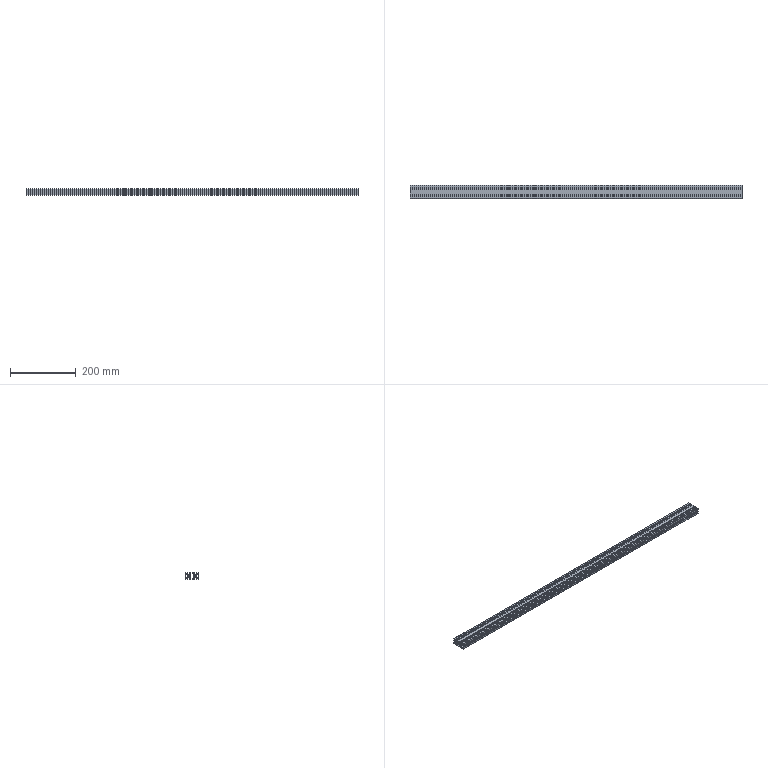Part | STEP file | 1 solid | 134 faces | box 1008 x 40 x 20 mm | volume 300919 mm3 | plane 126 | cylinder 8 | commonest cylinder face diameters 2 x4 5 x4